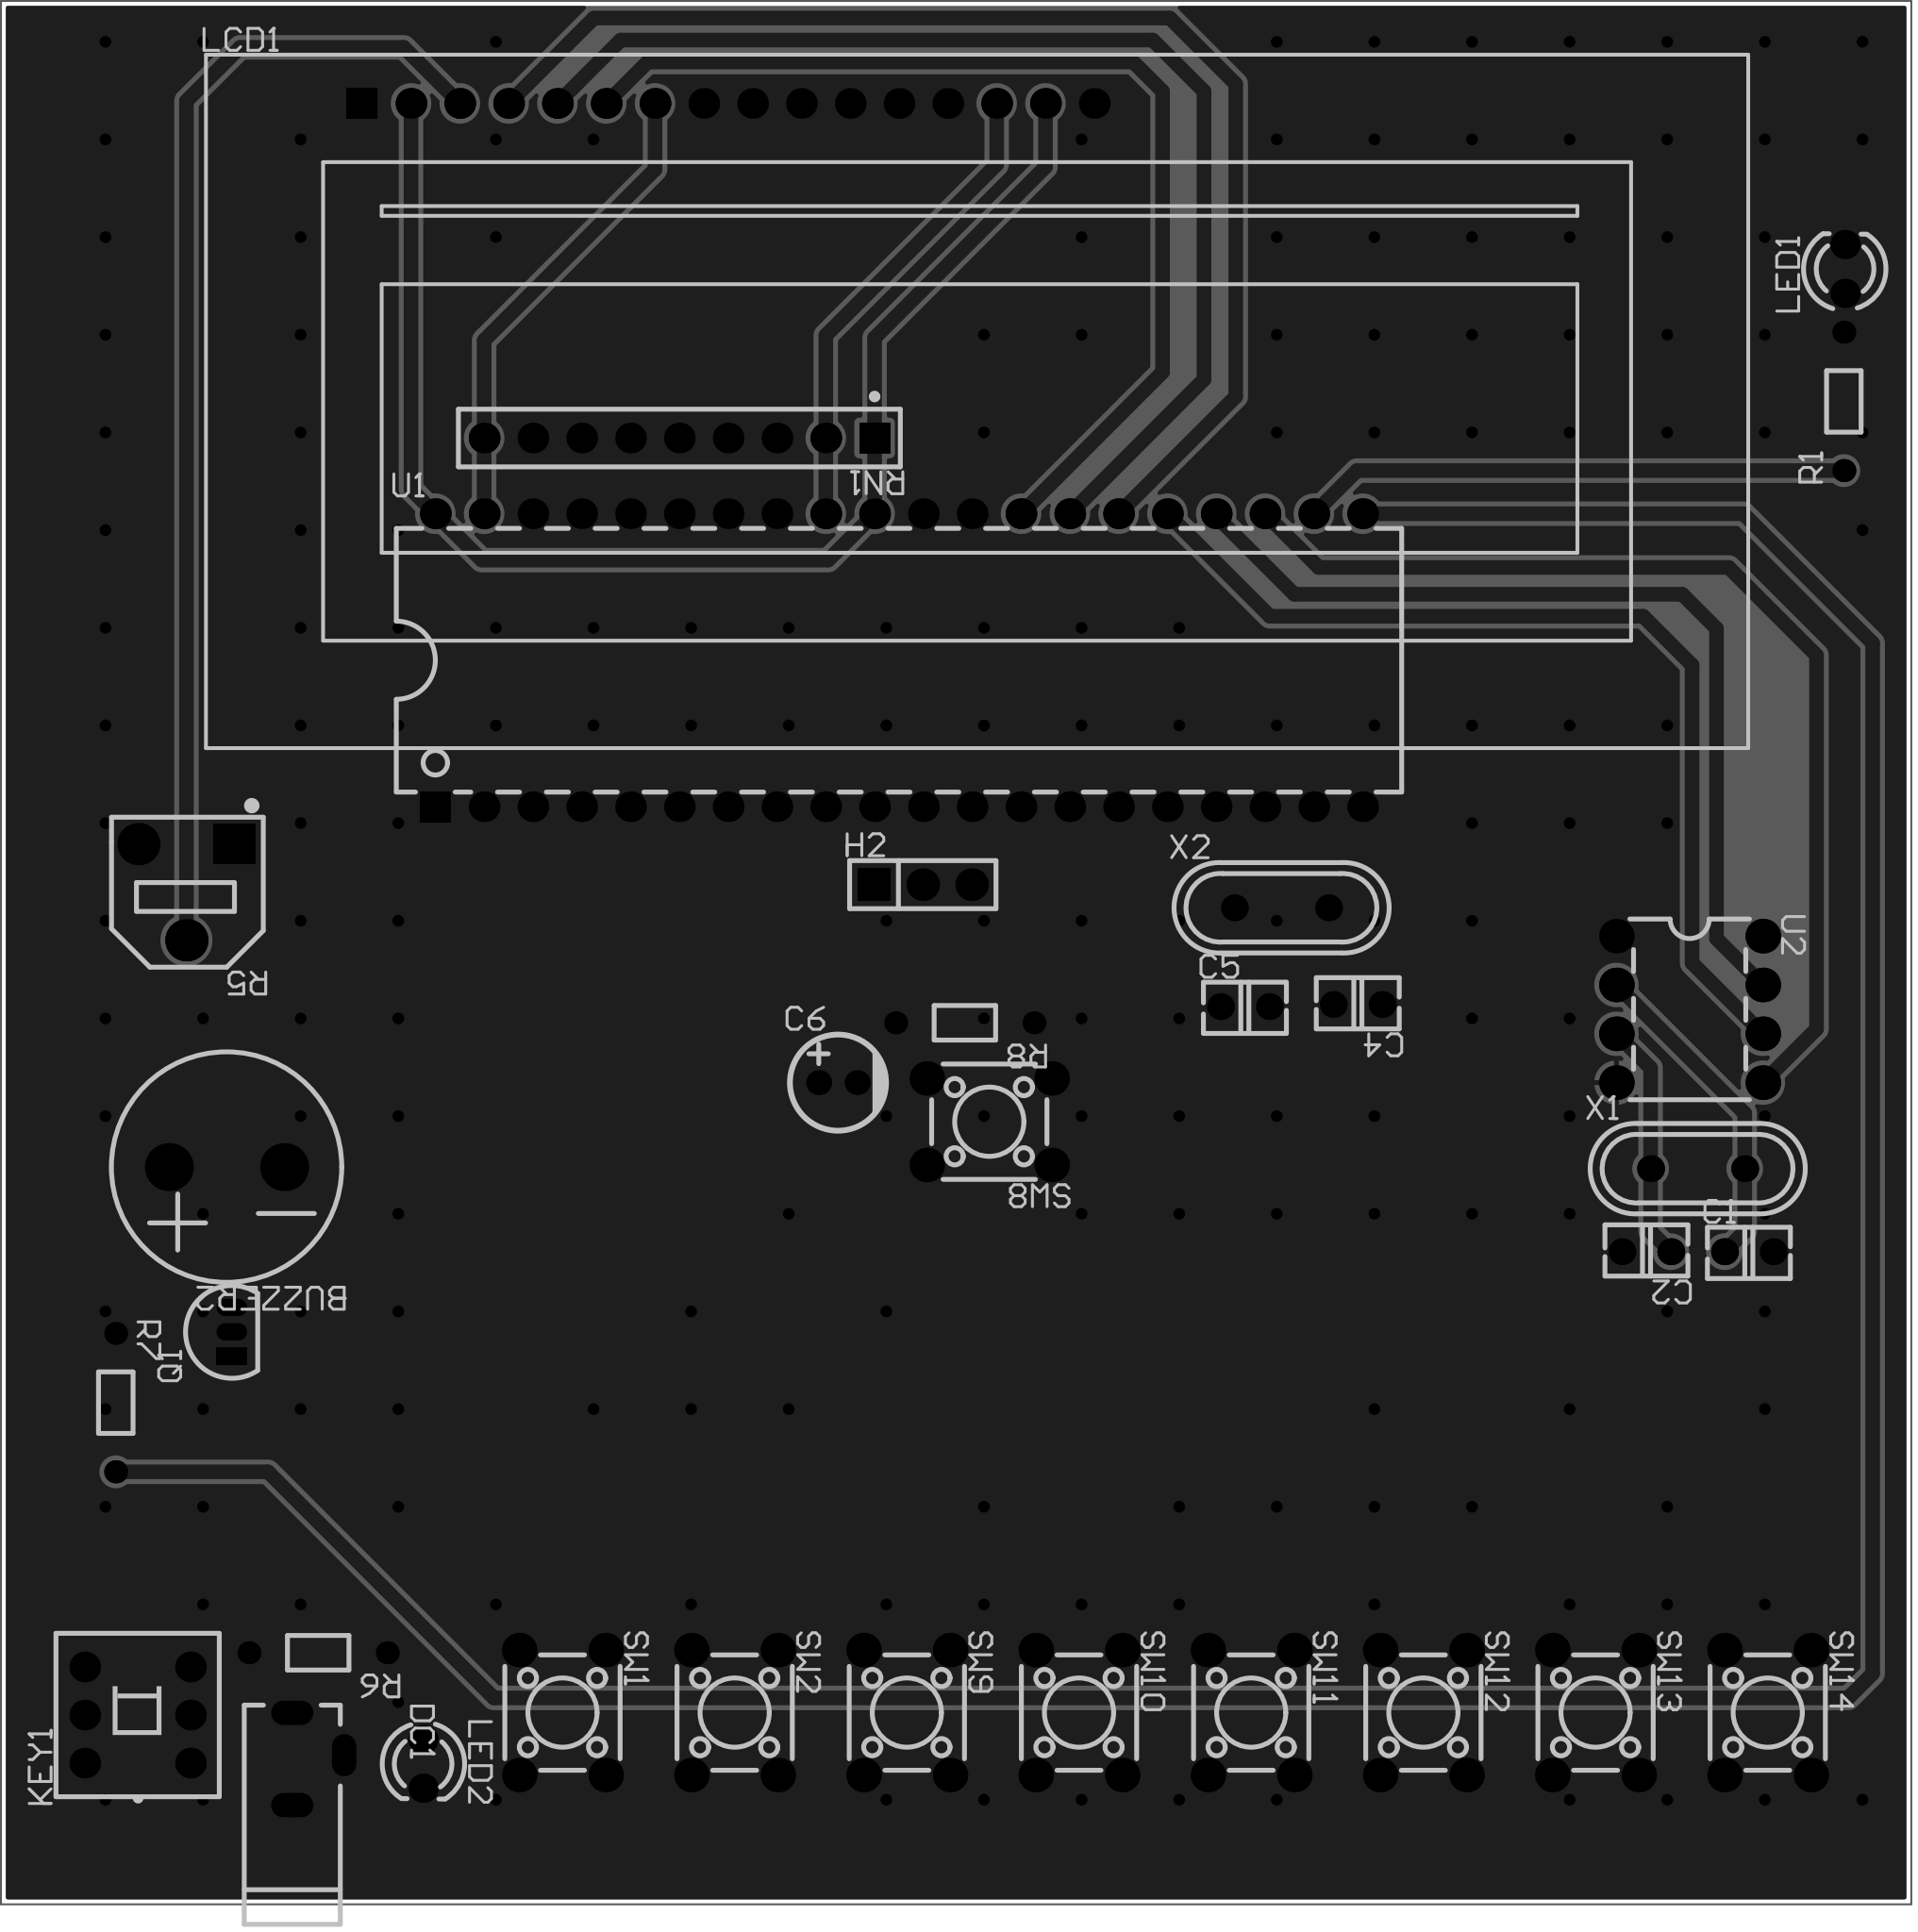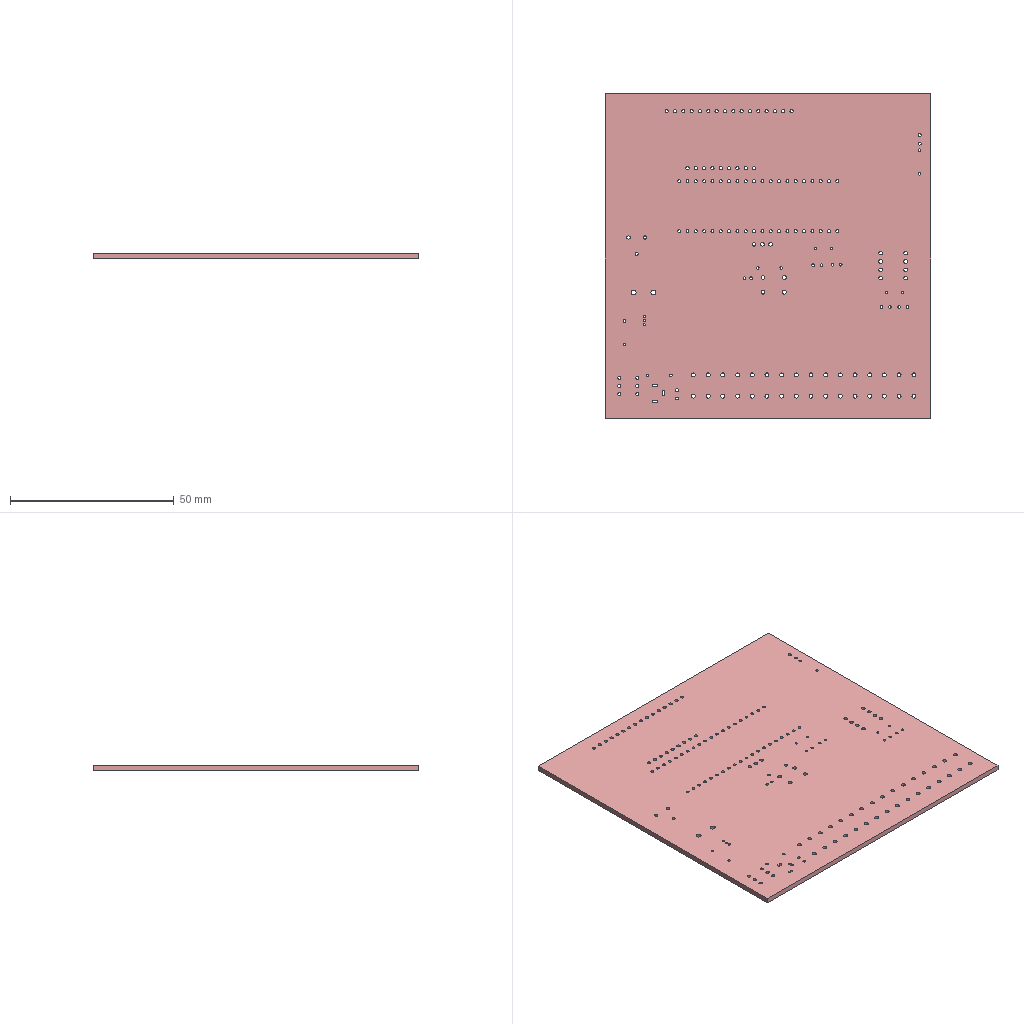Circuit board layout | Altium Designer | box 99.4 x 99 x 1.6 mm
Layer stack:
# Altium Designer layer stack of  (unit mm; dielectric type: 0 none, 1 core, 2 prepreg, 3 surface material)
index,name,kind,layer,copper_thickness_mm,dielectric_type,dielectric_thickness_mm,dielectric_material,dielectric_constant
0,Top Paste Mask Layer,other,,,,,,
1,Top Silkscreen Layer,other,,,,,,
2,Top Solder Mask Layer,dielectric,,,3,0.01,,3.3
3,Top Layer,copper,Top Layer,0.035,,,,
4,Dielectric1,dielectric,,,3,1.51,FR4,4.5
5,Bottom Layer,copper,Bottom Layer,0.035,,,,
6,Bottom Solder Mask Layer,dielectric,,,3,0.01,,3.3
7,Bottom Silkscreen Layer,other,,,,,,
8,Bottom Paste Mask Layer,other,,,,,,
# drill layer pairs: low layer,high layer
drill_pair,Top Layer,Bottom Layer
Part placement:
Designator,Comment,Layer,Footprint,Center-X(mm),Center-Y(mm),Rotation
BUZZER2,buzzer,TopLayer,BUZ-TH_BD12.0-P6.00-D0.9-RD,99.116,127.052,180
C4,22pF,TopLayer,CAP-TH_L3.8-W2.5-P2.54-D0.50,157.988,135.509,180
C5,22pF,TopLayer,CAP-TH_L3.8-W2.5-P2.54-D0.50,152.116,135.4,0
C6,10uF,TopLayer,CAP-TH_BD5.0-P2.00-D0.8-FD-10UF50VC110GL,130.937,131.445,0
H2,,TopLayer,HDR-TH_3P-P2.54-V-M,135.352,141.744,0
KEY1,Non-latching switch 8.5×8.5 silent,TopLayer,SW-TH_6P-L8.5-W8.5-P2.54,94.488,98.552,90
LCD1,HS1602A,TopLayer,LCD1602,125.226,182.378,0
LED2,,TopLayer,LED_TH-3mm,109.347,96.012,270
R7,10kΩ,TopLayer,Res_1/8W,93.351,114.801,270
R8,10kΩ,TopLayer,Res_1/8W,137.541,134.557,180
R5,10kΩ,TopLayer,RES-ADJ-SMD_RM065-V1,97.028,141.351,180
R6,1kΩ,TopLayer,Res_1/8W,103.886,101.791,180
SW8,,TopLayer,SW-TH_4P-L6.0-W6.0-P4.50-LS6.5,138.811,129.413,180
SW9,,TopLayer,SW-TH_4P-L6.0-W6.0-P4.50-LS6.5,134.52,98.679,270
SW10,,TopLayer,SW-TH_4P-L6.0-W6.0-P4.50-LS6.5,143.481,98.679,270
SW11,,TopLayer,SW-TH_4P-L6.0-W6.0-P4.50-LS6.5,152.442,98.679,270
SW12,,TopLayer,SW-TH_4P-L6.0-W6.0-P4.50-LS6.5,161.403,98.679,270
SW13,,TopLayer,SW-TH_4P-L6.0-W6.0-P4.50-LS6.5,170.363,98.679,270
SW14,,TopLayer,SW-TH_4P-L6.0-W6.0-P4.50-LS6.5,179.324,98.679,270
U1,STC89C52RC-40I-PDIP40,TopLayer,DIP-40_L52.0-W13.7-P2.54-LS15.2-BL,134.112,153.416,0
X2,11.059MHz,TopLayer,OSC-TH_L11.1-W4.7-P4.88,154.021,140.539,0
DC1,DC-002,TopLayer,DC-IN-TH_DC-3510,103.886,96.266,270
C1,1nF,TopLayer,CAP-TH_L3.8-W2.5-P2.54-D0.50,178.345,122.652,0
C2,1nF,TopLayer,CAP-TH_L3.8-W2.5-P2.54-D0.50,173.011,122.652,180
LED1,,TopLayer,LED_TH-3mm,183.347,173.768,90
Q1,,TopLayer,S8050_TO_92,99.392,118.48,90
R1,100,TopLayer,Res_1/8W,183.285,166.879,90
RN1,-,TopLayer,RES-ARRAY-TH_9P-P2.54-D1.0,122.682,164.973,180
SW1,,TopLayer,SW-TH_4P-L6.0-W6.0-P4.50-LS6.5,116.599,98.679,270
SW2,,TopLayer,SW-TH_4P-L6.0-W6.0-P4.50-LS6.5,125.559,98.679,270
U2,DS1302N(XBLW),TopLayer,PDIP-8_L9.3-W6.4-P2.54-LS7.6-BL,175.26,135.255,270
X1,11.059MHz,TopLayer,OSC-TH_L11.1-W4.7-P4.88,175.678,126.97,0
Pad and via stacks:
# Altium Designer via and pad stacks of  (unit mm). Each distinct definition once, with the count of objects using it.
# via: kind,start_layer,end_layer,hole_mm,diameter_mm,mode(0 simple;1 top-mid-bottom;2 full stack),diameter_per_layer,count,example_net
# pad: kind,layer,hole_mm,hole_type(0 round;1 square;2 slot),plating,top_size,top_shape(1 round;2 rect;3 octagon;9 rounded rect),mid_size,bottom_size,mode,footprint,size_per_layer,count,example
pad,Multi-Layer,1.5,0,plated,2.5x2.5,1,2.5x2.5,2.5x2.5,0,BUZ-TH_BD12.0-P6.00-D0.9-RD,,2,BUZZER2.1
pad,Multi-Layer,0.8,0,plated,1.4x1.4,1,1.4x1.4,1.4x1.4,0,CAP-TH_L3.8-W2.5-P2.54-D0.50,,8,C4.1
pad,Multi-Layer,0.8,0,plated,1.3x1.3,1,1.3x1.3,1.3x1.3,0,CAP-TH_BD5.0-P2.00-D0.8-FD-10UF50VC110GL,,2,C6.2
pad,Multi-Layer,1.1,0,plated,1.7x1.7,2,1.7x1.7,1.7x1.7,0,HDR-TH_3P-P2.54-V-M,,1,H2.1
pad,Multi-Layer,1.1,0,plated,1.7x1.7,1,1.7x1.7,1.7x1.7,0,HDR-TH_3P-P2.54-V-M,,2,H2.2
pad,Multi-Layer,1,0,plated,1.6x1.6,1,1.6x1.6,1.6x1.6,0,SW-TH_6P-L8.5-W8.5-P2.54,,6,KEY1.4
pad,Multi-Layer,1,0,plated,1.6x1.6,1,1.6x1.6,1.6x1.6,0,LCD1602,,15,LCD1.16
pad,Multi-Layer,1,0,plated,1.6x1.6,2,1.6x1.6,1.6x1.6,0,LCD1602,,1,LCD1.1
pad,Multi-Layer,0.9144,0,plated,1.524x1.524,1,1.524x1.524,1.524x1.524,0,LED_TH-3mm,,4,LED2.1
pad,Multi-Layer,0.8001,0,plated,1.199x1.199,1,1.199x1.199,1.199x1.199,0,Res_1/8W,,8,R7.1
pad,Multi-Layer,1,0,plated,2.2x2.1,2,2.2x2.1,2.2x2.1,0,RES-ADJ-SMD_RM065-V1,,1,R5.1
pad,Multi-Layer,1,0,plated,2.2x2.2,1,2.2x2.2,2.2x2.2,0,RES-ADJ-SMD_RM065-V1,,2,R5.3
pad,Multi-Layer,1.2,0,plated,1.8x1.8,1,1.8x1.8,1.8x1.8,0,SW-TH_4P-L6.0-W6.0-P4.50-LS6.5,,36,SW8.1
pad,Multi-Layer,0.889,0,plated,1.6x1.6,1,1.6x1.6,1.6x1.6,0,DIP-40_L52.0-W13.7-P2.54-LS15.2-BL,,39,U1.31
pad,Multi-Layer,0.889,0,plated,1.6x1.6,2,1.6x1.6,1.6x1.6,0,DIP-40_L52.0-W13.7-P2.54-LS15.2-BL,,1,U1.1
pad,Multi-Layer,0.7,0,plated,1.4x1.4,1,1.4x1.4,1.4x1.4,0,OSC-TH_L11.1-W4.7-P4.88,,4,X2.1
pad,Multi-Layer,0.8,2,plated,2.2x1.27,1,2.2x1.27,2.2x1.27,0,DC-IN-TH_DC-3510,,3,DC1.3
pad,Multi-Layer,0.701,0,plated,0.8992x1.6,2,0.8992x1.6,0.8992x1.6,0,S8050_TO_92,,1,Q1.1
pad,Multi-Layer,0.701,0,plated,0.8992x1.6,1,0.8992x1.6,0.8992x1.6,0,S8050_TO_92,,2,Q1.2
pad,Multi-Layer,1,0,plated,1.6x1.6,2,1.6x1.6,1.6x1.6,0,RES-ARRAY-TH_9P-P2.54-D1.0,,1,RN1.1
pad,Multi-Layer,1,0,plated,1.6x1.6,1,1.6x1.6,1.6x1.6,0,RES-ARRAY-TH_9P-P2.54-D1.0,,8,RN1.2
pad,Multi-Layer,1.1,0,plated,1.8x1.8,1,1.8x1.8,1.8x1.8,0,PDIP-8_L9.3-W6.4-P2.54-LS7.6-BL,,8,U2.1
via,Top Layer,Bottom Layer,0.3048,0.61,0,,181,GND
Copper pours:
name,layer,net,type(0 solid;1 hatched;2 none)
Bottom Layer-GND,Bottom Layer,GND,0
Top Layer-GND,Top Layer,GND,0
Design rules, without the lines most boards share:
# Altium Designer design rules of  (exported by Altium Designer, unit mm)
# columns: name | kind | enabled | priority | scope1 | scope2 | descriptor | typed fields (field=value)
creepage | 65 | enabled | 1 | All | All | Creepage Distance Constraint =(0mil) (All),(All) |